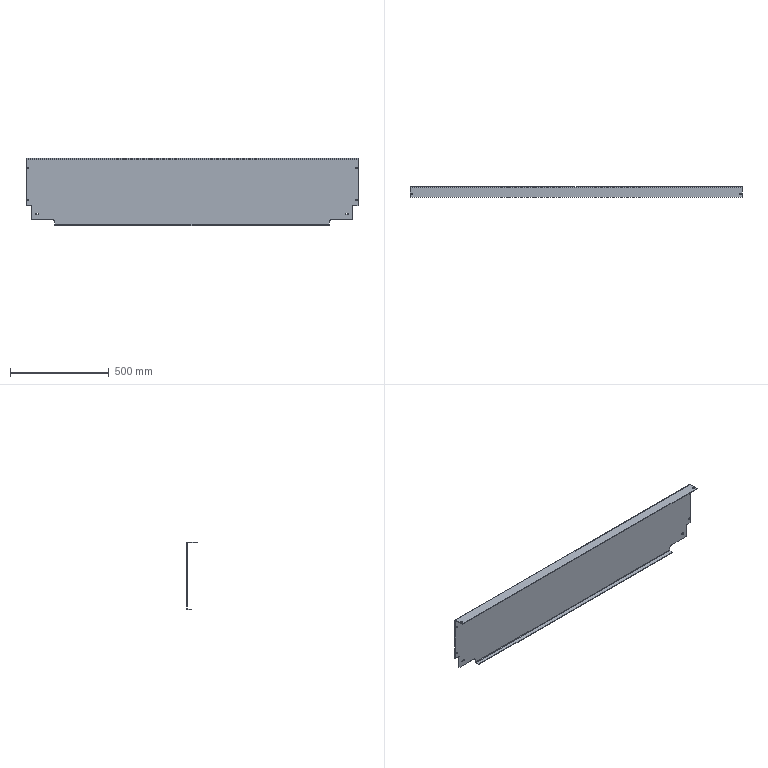Part | SolidWorks | features BaseBody 1 | 1 solid | 70 faces | box 1680 x 53 x 340 mm | volume 2004466 mm3 | plane 42 | cylinder 28 | commonest cylinder face diameters 7 x18 3 x4 4 x2 10 x2 30 x2